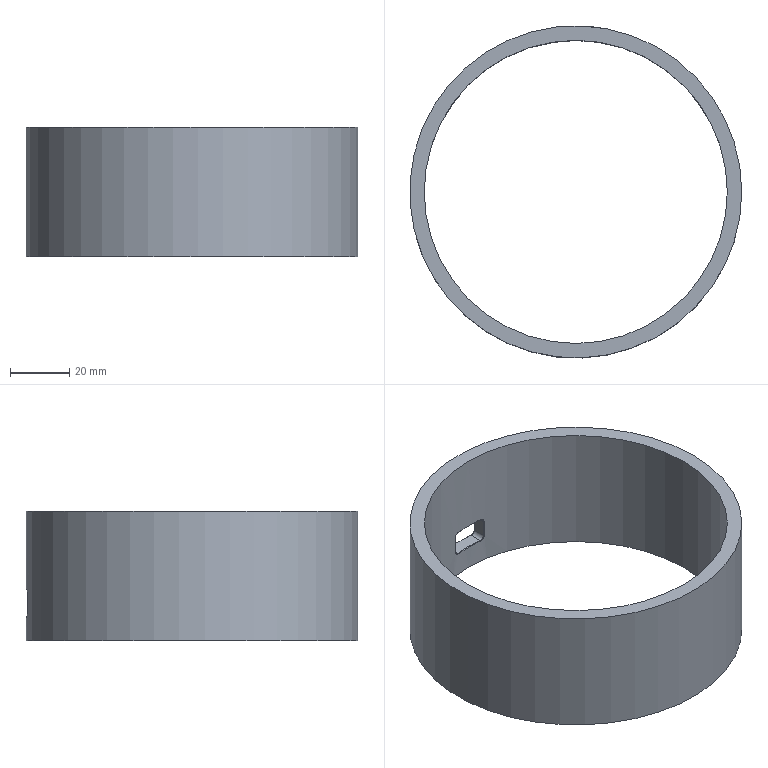Part | 1 solid | 28 faces | box 112.5 x 112.5 x 44 mm | volume 72321 mm3 | plane 10 | spline 8 | cylinder 6 | cone 4 | commonest cylinder face diameters 3 x4 102.7 x1 112.5 x1
STEP:
#1=CARTESIAN_POINT('',(-7.25,55.781,-28.5));
#2=VERTEX_POINT('',#1);
#3=CARTESIAN_POINT('',(-7.25,55.781,-34.));
#4=VERTEX_POINT('',#3);
#5=CARTESIAN_POINT('',(-7.25,55.781,0.));
#6=DIRECTION('',(0.,0.,-1.));
#7=VECTOR('',#6,1000.);
#8=LINE('',#5,#7);
#9=EDGE_CURVE('',#2,#4,#8,.T.);
#10=ORIENTED_EDGE('',*,*,#9,.T.);
#11=CARTESIAN_POINT('',(-5.292,56.001,-35.943));
#12=VERTEX_POINT('',#11);
#13=CARTESIAN_POINT('',(-7.25,55.781,-34.));
#14=CARTESIAN_POINT('',(-7.25,55.781,-35.034));
#15=CARTESIAN_POINT('',(-6.327,55.903,-35.945));
#16=CARTESIAN_POINT('',(-5.292,56.001,-35.943));
#17=B_SPLINE_CURVE_WITH_KNOTS('',3,(#13,#14,#15,#16),.UNSPECIFIED.,.F.,.F.,(4,4),(0.,1.),.UNSPECIFIED.);
#18=EDGE_CURVE('',#4,#12,#17,.T.);
#19=ORIENTED_EDGE('',*,*,#18,.T.);
#20=CARTESIAN_POINT('',(5.292,56.001,-35.943));
#21=VERTEX_POINT('',#20);
#22=CARTESIAN_POINT('',(0.,0.,-35.943));
#23=DIRECTION('',(0.,0.,1.));
#24=DIRECTION('',(1.,0.,0.));
#25=AXIS2_PLACEMENT_3D('',#22,#23,#24);
#26=CIRCLE('',#25,56.25);
#27=EDGE_CURVE('',#12,#21,#26,.F.);
#28=ORIENTED_EDGE('',*,*,#27,.T.);
#29=CARTESIAN_POINT('',(7.25,55.781,-34.));
#30=VERTEX_POINT('',#29);
#31=CARTESIAN_POINT('',(5.292,56.001,-35.943));
#32=CARTESIAN_POINT('',(6.33,55.902,-35.943));
#33=CARTESIAN_POINT('',(7.252,55.781,-35.032));
#34=CARTESIAN_POINT('',(7.25,55.781,-34.));
#35=B_SPLINE_CURVE_WITH_KNOTS('',3,(#31,#32,#33,#34),.UNSPECIFIED.,.F.,.F.,(4,4),(0.,1.),.UNSPECIFIED.);
#36=EDGE_CURVE('',#21,#30,#35,.T.);
#37=ORIENTED_EDGE('',*,*,#36,.T.);
#38=CARTESIAN_POINT('',(7.25,55.781,-28.5));
#39=VERTEX_POINT('',#38);
#40=CARTESIAN_POINT('',(7.25,55.781,0.));
#41=DIRECTION('',(0.,0.,-1.));
#42=VECTOR('',#41,1000.);
#43=LINE('',#40,#42);
#44=EDGE_CURVE('',#30,#39,#43,.F.);
#45=ORIENTED_EDGE('',*,*,#44,.T.);
#46=CARTESIAN_POINT('',(5.292,56.001,-26.557));
#47=VERTEX_POINT('',#46);
#48=CARTESIAN_POINT('',(7.25,55.781,-28.5));
#49=CARTESIAN_POINT('',(7.25,55.781,-27.466));
#50=CARTESIAN_POINT('',(6.327,55.903,-26.555));
#51=CARTESIAN_POINT('',(5.292,56.001,-26.557));
#52=B_SPLINE_CURVE_WITH_KNOTS('',3,(#48,#49,#50,#51),.UNSPECIFIED.,.F.,.F.,(4,4),(0.,1.),.UNSPECIFIED.);
#53=EDGE_CURVE('',#39,#47,#52,.T.);
#54=ORIENTED_EDGE('',*,*,#53,.T.);
#55=CARTESIAN_POINT('',(-5.292,56.001,-26.557));
#56=VERTEX_POINT('',#55);
#57=CARTESIAN_POINT('',(0.,0.,-26.557));
#58=DIRECTION('',(0.,0.,-1.));
#59=DIRECTION('',(-1.,0.,0.));
#60=AXIS2_PLACEMENT_3D('',#57,#58,#59);
#61=CIRCLE('',#60,56.25);
#62=EDGE_CURVE('',#47,#56,#61,.F.);
#63=ORIENTED_EDGE('',*,*,#62,.T.);
#64=CARTESIAN_POINT('',(-5.292,56.001,-26.557));
#65=CARTESIAN_POINT('',(-6.33,55.902,-26.557));
#66=CARTESIAN_POINT('',(-7.252,55.781,-27.468));
#67=CARTESIAN_POINT('',(-7.25,55.781,-28.5));
#68=B_SPLINE_CURVE_WITH_KNOTS('',3,(#64,#65,#66,#67),.UNSPECIFIED.,.F.,.F.,(4,4),(0.,1.),.UNSPECIFIED.);
#69=EDGE_CURVE('',#56,#2,#68,.T.);
#70=ORIENTED_EDGE('',*,*,#69,.T.);
#71=EDGE_LOOP('',(#10,#19,#28,#37,#45,#54,#63,#70));
#72=FACE_BOUND('',#71,.T.);
#73=CARTESIAN_POINT('',(56.25,0.,0.));
#74=VERTEX_POINT('',#73);
#75=CARTESIAN_POINT('',(0.,0.,0.));
#76=DIRECTION('',(0.,0.,1.));
#77=DIRECTION('',(1.,0.,0.));
#78=AXIS2_PLACEMENT_3D('',#75,#76,#77);
#79=CIRCLE('',#78,56.25);
#80=EDGE_CURVE('',#74,#74,#79,.T.);
#81=ORIENTED_EDGE('',*,*,#80,.F.);
#82=EDGE_LOOP('',(#81));
#83=FACE_BOUND('',#82,.T.);
#84=CARTESIAN_POINT('',(56.25,0.,-44.));
#85=VERTEX_POINT('',#84);
#86=CARTESIAN_POINT('',(0.,0.,-44.));
#87=DIRECTION('',(0.,0.,1.));
#88=DIRECTION('',(1.,0.,0.));
#89=AXIS2_PLACEMENT_3D('',#86,#87,#88);
#90=CIRCLE('',#89,56.25);
#91=EDGE_CURVE('',#85,#85,#90,.T.);
#92=ORIENTED_EDGE('',*,*,#91,.T.);
#93=EDGE_LOOP('',(#92));
#94=FACE_BOUND('',#93,.T.);
#95=CARTESIAN_POINT('',(0.,0.,0.));
#96=DIRECTION('',(0.,0.,-1.));
#97=DIRECTION('',(-1.,0.,0.));
#98=AXIS2_PLACEMENT_3D('',#95,#96,#97);
#99=CYLINDRICAL_SURFACE('',#98,56.25);
#100=ADVANCED_FACE('',(#72,#83,#94),#99,.T.);
#101=CARTESIAN_POINT('',(-6.923,50.881,-34.));
#102=VERTEX_POINT('',#101);
#103=CARTESIAN_POINT('',(-6.923,50.881,-28.5));
#104=VERTEX_POINT('',#103);
#105=CARTESIAN_POINT('',(-6.923,50.881,0.));
#106=DIRECTION('',(0.,0.,-1.));
#107=VECTOR('',#106,1000.);
#108=LINE('',#105,#107);
#109=EDGE_CURVE('',#102,#104,#108,.F.);
#110=ORIENTED_EDGE('',*,*,#109,.T.);
#111=CARTESIAN_POINT('',(-5.23,51.083,-26.8));
#112=VERTEX_POINT('',#111);
#113=CARTESIAN_POINT('',(-6.923,50.881,-28.5));
#114=CARTESIAN_POINT('',(-6.924,50.881,-27.597));
#115=CARTESIAN_POINT('',(-6.126,50.991,-26.801));
#116=CARTESIAN_POINT('',(-5.23,51.083,-26.8));
#117=B_SPLINE_CURVE_WITH_KNOTS('',3,(#113,#114,#115,#116),.UNSPECIFIED.,.F.,.F.,(4,4),(0.,1.),.UNSPECIFIED.);
#118=EDGE_CURVE('',#104,#112,#117,.T.);
#119=ORIENTED_EDGE('',*,*,#118,.T.);
#120=CARTESIAN_POINT('',(5.23,51.083,-26.8));
#121=VERTEX_POINT('',#120);
#122=CARTESIAN_POINT('',(0.,0.,-26.8));
#123=DIRECTION('',(0.,0.,-1.));
#124=DIRECTION('',(-1.,0.,0.));
#125=AXIS2_PLACEMENT_3D('',#122,#123,#124);
#126=CIRCLE('',#125,51.35);
#127=EDGE_CURVE('',#112,#121,#126,.T.);
#128=ORIENTED_EDGE('',*,*,#127,.T.);
#129=CARTESIAN_POINT('',(6.923,50.881,-28.5));
#130=VERTEX_POINT('',#129);
#131=CARTESIAN_POINT('',(5.23,51.083,-26.8));
#132=CARTESIAN_POINT('',(6.118,50.992,-26.797));
#133=CARTESIAN_POINT('',(6.923,50.881,-27.596));
#134=CARTESIAN_POINT('',(6.923,50.881,-28.5));
#135=B_SPLINE_CURVE_WITH_KNOTS('',3,(#131,#132,#133,#134),.UNSPECIFIED.,.F.,.F.,(4,4),(0.,1.),.UNSPECIFIED.);
#136=EDGE_CURVE('',#121,#130,#135,.T.);
#137=ORIENTED_EDGE('',*,*,#136,.T.);
#138=CARTESIAN_POINT('',(6.923,50.881,-34.));
#139=VERTEX_POINT('',#138);
#140=CARTESIAN_POINT('',(6.923,50.881,0.));
#141=DIRECTION('',(0.,0.,-1.));
#142=VECTOR('',#141,1000.);
#143=LINE('',#140,#142);
#144=EDGE_CURVE('',#130,#139,#143,.T.);
#145=ORIENTED_EDGE('',*,*,#144,.T.);
#146=CARTESIAN_POINT('',(5.23,51.083,-35.7));
#147=VERTEX_POINT('',#146);
#148=CARTESIAN_POINT('',(6.923,50.881,-34.));
#149=CARTESIAN_POINT('',(6.924,50.881,-34.903));
#150=CARTESIAN_POINT('',(6.126,50.991,-35.699));
#151=CARTESIAN_POINT('',(5.23,51.083,-35.7));
#152=B_SPLINE_CURVE_WITH_KNOTS('',3,(#148,#149,#150,#151),.UNSPECIFIED.,.F.,.F.,(4,4),(0.,1.),.UNSPECIFIED.);
#153=EDGE_CURVE('',#139,#147,#152,.T.);
#154=ORIENTED_EDGE('',*,*,#153,.T.);
#155=CARTESIAN_POINT('',(-5.23,51.083,-35.7));
#156=VERTEX_POINT('',#155);
#157=CARTESIAN_POINT('',(0.,0.,-35.7));
#158=DIRECTION('',(0.,0.,1.));
#159=DIRECTION('',(1.,0.,0.));
#160=AXIS2_PLACEMENT_3D('',#157,#158,#159);
#161=CIRCLE('',#160,51.35);
#162=EDGE_CURVE('',#147,#156,#161,.T.);
#163=ORIENTED_EDGE('',*,*,#162,.T.);
#164=CARTESIAN_POINT('',(-5.23,51.083,-35.7));
#165=CARTESIAN_POINT('',(-6.118,50.992,-35.703));
#166=CARTESIAN_POINT('',(-6.923,50.881,-34.904));
#167=CARTESIAN_POINT('',(-6.923,50.881,-34.));
#168=B_SPLINE_CURVE_WITH_KNOTS('',3,(#164,#165,#166,#167),.UNSPECIFIED.,.F.,.F.,(4,4),(0.,1.),.UNSPECIFIED.);
#169=EDGE_CURVE('',#156,#102,#168,.T.);
#170=ORIENTED_EDGE('',*,*,#169,.T.);
#171=EDGE_LOOP('',(#110,#119,#128,#137,#145,#154,#163,#170));
#172=FACE_BOUND('',#171,.T.);
#173=CARTESIAN_POINT('',(51.35,0.,0.));
#174=VERTEX_POINT('',#173);
#175=CARTESIAN_POINT('',(0.,0.,0.));
#176=DIRECTION('',(0.,0.,1.));
#177=DIRECTION('',(1.,0.,0.));
#178=AXIS2_PLACEMENT_3D('',#175,#176,#177);
#179=CIRCLE('',#178,51.35);
#180=EDGE_CURVE('',#174,#174,#179,.T.);
#181=ORIENTED_EDGE('',*,*,#180,.T.);
#182=EDGE_LOOP('',(#181));
#183=FACE_BOUND('',#182,.T.);
#184=CARTESIAN_POINT('',(51.35,0.,-44.));
#185=VERTEX_POINT('',#184);
#186=CARTESIAN_POINT('',(0.,0.,-44.));
#187=DIRECTION('',(0.,0.,1.));
#188=DIRECTION('',(1.,0.,0.));
#189=AXIS2_PLACEMENT_3D('',#186,#187,#188);
#190=CIRCLE('',#189,51.35);
#191=EDGE_CURVE('',#185,#185,#190,.T.);
#192=ORIENTED_EDGE('',*,*,#191,.F.);
#193=EDGE_LOOP('',(#192));
#194=FACE_BOUND('',#193,.T.);
#195=CARTESIAN_POINT('',(0.,0.,0.));
#196=DIRECTION('',(0.,0.,-1.));
#197=DIRECTION('',(-1.,0.,0.));
#198=AXIS2_PLACEMENT_3D('',#195,#196,#197);
#199=CYLINDRICAL_SURFACE('',#198,51.35);
#200=ADVANCED_FACE('',(#172,#183,#194),#199,.F.);
#201=ORIENTED_EDGE('',*,*,#80,.T.);
#202=EDGE_LOOP('',(#201));
#203=FACE_BOUND('',#202,.T.);
#204=ORIENTED_EDGE('',*,*,#180,.F.);
#205=EDGE_LOOP('',(#204));
#206=FACE_BOUND('',#205,.T.);
#207=CARTESIAN_POINT('',(0.,0.,0.));
#208=DIRECTION('',(0.,0.,1.));
#209=DIRECTION('',(1.,0.,0.));
#210=AXIS2_PLACEMENT_3D('',#207,#208,#209);
#211=PLANE('',#210);
#212=ADVANCED_FACE('',(#203,#206),#211,.T.);
#213=ORIENTED_EDGE('',*,*,#91,.F.);
#214=EDGE_LOOP('',(#213));
#215=FACE_BOUND('',#214,.T.);
#216=ORIENTED_EDGE('',*,*,#191,.T.);
#217=EDGE_LOOP('',(#216));
#218=FACE_BOUND('',#217,.T.);
#219=CARTESIAN_POINT('',(0.,0.,-44.));
#220=DIRECTION('',(0.,0.,1.));
#221=DIRECTION('',(1.,0.,0.));
#222=AXIS2_PLACEMENT_3D('',#219,#220,#221);
#223=PLANE('',#222);
#224=ADVANCED_FACE('',(#215,#218),#223,.F.);
#225=CARTESIAN_POINT('',(-6.75,55.341,-28.5));
#226=VERTEX_POINT('',#225);
#227=CARTESIAN_POINT('',(-6.75,51.079,-28.5));
#228=VERTEX_POINT('',#227);
#229=CARTESIAN_POINT('',(-6.75,50.904,-28.5));
#230=DIRECTION('',(0.,1.,0.));
#231=VECTOR('',#230,1000.);
#232=LINE('',#229,#231);
#233=EDGE_CURVE('',#226,#228,#232,.F.);
#234=ORIENTED_EDGE('',*,*,#233,.T.);
#235=CARTESIAN_POINT('',(-6.75,51.079,-34.));
#236=VERTEX_POINT('',#235);
#237=CARTESIAN_POINT('',(-6.75,51.079,-35.5));
#238=DIRECTION('',(0.,0.,-1.));
#239=VECTOR('',#238,1000.);
#240=LINE('',#237,#239);
#241=EDGE_CURVE('',#228,#236,#240,.T.);
#242=ORIENTED_EDGE('',*,*,#241,.T.);
#243=CARTESIAN_POINT('',(-6.75,55.341,-34.));
#244=VERTEX_POINT('',#243);
#245=CARTESIAN_POINT('',(-6.75,55.844,-34.));
#246=DIRECTION('',(0.,1.,0.));
#247=VECTOR('',#246,1000.);
#248=LINE('',#245,#247);
#249=EDGE_CURVE('',#236,#244,#248,.T.);
#250=ORIENTED_EDGE('',*,*,#249,.T.);
#251=CARTESIAN_POINT('',(-6.75,55.341,-28.5));
#252=DIRECTION('',(0.,0.,1.));
#253=VECTOR('',#252,1000.);
#254=LINE('',#251,#253);
#255=EDGE_CURVE('',#244,#226,#254,.T.);
#256=ORIENTED_EDGE('',*,*,#255,.T.);
#257=EDGE_LOOP('',(#234,#242,#250,#256));
#258=FACE_BOUND('',#257,.T.);
#259=CARTESIAN_POINT('',(-6.75,56.25,-35.5));
#260=DIRECTION('',(1.,0.,0.));
#261=DIRECTION('',(0.,0.,-1.));
#262=AXIS2_PLACEMENT_3D('',#259,#260,#261);
#263=PLANE('',#262);
#264=ADVANCED_FACE('',(#258),#263,.T.);
#265=CARTESIAN_POINT('',(5.25,55.559,-27.));
#266=VERTEX_POINT('',#265);
#267=CARTESIAN_POINT('',(5.25,51.282,-27.));
#268=VERTEX_POINT('',#267);
#269=CARTESIAN_POINT('',(5.25,50.904,-27.));
#270=DIRECTION('',(0.,1.,0.));
#271=VECTOR('',#270,1000.);
#272=LINE('',#269,#271);
#273=EDGE_CURVE('',#266,#268,#272,.F.);
#274=ORIENTED_EDGE('',*,*,#273,.T.);
#275=CARTESIAN_POINT('',(-5.25,51.282,-27.));
#276=VERTEX_POINT('',#275);
#277=CARTESIAN_POINT('',(0.,0.,-27.));
#278=DIRECTION('',(0.,0.,-1.));
#279=DIRECTION('',(-1.,0.,0.));
#280=AXIS2_PLACEMENT_3D('',#277,#278,#279);
#281=CIRCLE('',#280,51.55);
#282=EDGE_CURVE('',#268,#276,#281,.F.);
#283=ORIENTED_EDGE('',*,*,#282,.T.);
#284=CARTESIAN_POINT('',(-5.25,55.559,-27.));
#285=VERTEX_POINT('',#284);
#286=CARTESIAN_POINT('',(-5.25,55.844,-27.));
#287=DIRECTION('',(0.,1.,0.));
#288=VECTOR('',#287,1000.);
#289=LINE('',#286,#288);
#290=EDGE_CURVE('',#276,#285,#289,.T.);
#291=ORIENTED_EDGE('',*,*,#290,.T.);
#292=CARTESIAN_POINT('',(0.,0.,-27.));
#293=DIRECTION('',(0.,0.,-1.));
#294=DIRECTION('',(-1.,0.,0.));
#295=AXIS2_PLACEMENT_3D('',#292,#293,#294);
#296=CIRCLE('',#295,55.807);
#297=EDGE_CURVE('',#285,#266,#296,.T.);
#298=ORIENTED_EDGE('',*,*,#297,.T.);
#299=EDGE_LOOP('',(#274,#283,#291,#298));
#300=FACE_BOUND('',#299,.T.);
#301=CARTESIAN_POINT('',(-6.75,56.25,-27.));
#302=DIRECTION('',(0.,0.,-1.));
#303=DIRECTION('',(-1.,0.,0.));
#304=AXIS2_PLACEMENT_3D('',#301,#302,#303);
#305=PLANE('',#304);
#306=ADVANCED_FACE('',(#300),#305,.T.);
#307=CARTESIAN_POINT('',(6.75,55.341,-34.));
#308=VERTEX_POINT('',#307);
#309=CARTESIAN_POINT('',(6.75,51.079,-34.));
#310=VERTEX_POINT('',#309);
#311=CARTESIAN_POINT('',(6.75,50.904,-34.));
#312=DIRECTION('',(0.,1.,0.));
#313=VECTOR('',#312,1000.);
#314=LINE('',#311,#313);
#315=EDGE_CURVE('',#308,#310,#314,.F.);
#316=ORIENTED_EDGE('',*,*,#315,.T.);
#317=CARTESIAN_POINT('',(6.75,51.079,-28.5));
#318=VERTEX_POINT('',#317);
#319=CARTESIAN_POINT('',(6.75,51.079,-27.));
#320=DIRECTION('',(0.,0.,1.));
#321=VECTOR('',#320,1000.);
#322=LINE('',#319,#321);
#323=EDGE_CURVE('',#310,#318,#322,.T.);
#324=ORIENTED_EDGE('',*,*,#323,.T.);
#325=CARTESIAN_POINT('',(6.75,55.341,-28.5));
#326=VERTEX_POINT('',#325);
#327=CARTESIAN_POINT('',(6.75,55.844,-28.5));
#328=DIRECTION('',(0.,1.,0.));
#329=VECTOR('',#328,1000.);
#330=LINE('',#327,#329);
#331=EDGE_CURVE('',#318,#326,#330,.T.);
#332=ORIENTED_EDGE('',*,*,#331,.T.);
#333=CARTESIAN_POINT('',(6.75,55.341,-34.));
#334=DIRECTION('',(0.,0.,-1.));
#335=VECTOR('',#334,1000.);
#336=LINE('',#333,#335);
#337=EDGE_CURVE('',#326,#308,#336,.T.);
#338=ORIENTED_EDGE('',*,*,#337,.T.);
#339=EDGE_LOOP('',(#316,#324,#332,#338));
#340=FACE_BOUND('',#339,.T.);
#341=CARTESIAN_POINT('',(6.75,56.25,-27.));
#342=DIRECTION('',(-1.,0.,0.));
#343=DIRECTION('',(0.,0.,1.));
#344=AXIS2_PLACEMENT_3D('',#341,#342,#343);
#345=PLANE('',#344);
#346=ADVANCED_FACE('',(#340),#345,.T.);
#347=CARTESIAN_POINT('',(-5.25,55.559,-35.5));
#348=VERTEX_POINT('',#347);
#349=CARTESIAN_POINT('',(-5.25,51.282,-35.5));
#350=VERTEX_POINT('',#349);
#351=CARTESIAN_POINT('',(-5.25,50.904,-35.5));
#352=DIRECTION('',(0.,1.,0.));
#353=VECTOR('',#352,1000.);
#354=LINE('',#351,#353);
#355=EDGE_CURVE('',#348,#350,#354,.F.);
#356=ORIENTED_EDGE('',*,*,#355,.T.);
#357=CARTESIAN_POINT('',(5.25,51.282,-35.5));
#358=VERTEX_POINT('',#357);
#359=CARTESIAN_POINT('',(0.,0.,-35.5));
#360=DIRECTION('',(0.,0.,1.));
#361=DIRECTION('',(1.,0.,0.));
#362=AXIS2_PLACEMENT_3D('',#359,#360,#361);
#363=CIRCLE('',#362,51.55);
#364=EDGE_CURVE('',#350,#358,#363,.F.);
#365=ORIENTED_EDGE('',*,*,#364,.T.);
#366=CARTESIAN_POINT('',(5.25,55.559,-35.5));
#367=VERTEX_POINT('',#366);
#368=CARTESIAN_POINT('',(5.25,55.844,-35.5));
#369=DIRECTION('',(0.,1.,0.));
#370=VECTOR('',#369,1000.);
#371=LINE('',#368,#370);
#372=EDGE_CURVE('',#358,#367,#371,.T.);
#373=ORIENTED_EDGE('',*,*,#372,.T.);
#374=CARTESIAN_POINT('',(0.,0.,-35.5));
#375=DIRECTION('',(0.,0.,1.));
#376=DIRECTION('',(1.,0.,0.));
#377=AXIS2_PLACEMENT_3D('',#374,#375,#376);
#378=CIRCLE('',#377,55.807);
#379=EDGE_CURVE('',#367,#348,#378,.T.);
#380=ORIENTED_EDGE('',*,*,#379,.T.);
#381=EDGE_LOOP('',(#356,#365,#373,#380));
#382=FACE_BOUND('',#381,.T.);
#383=CARTESIAN_POINT('',(6.75,56.25,-35.5));
#384=DIRECTION('',(0.,0.,1.));
#385=DIRECTION('',(1.,0.,0.));
#386=AXIS2_PLACEMENT_3D('',#383,#384,#385);
#387=PLANE('',#386);
#388=ADVANCED_FACE('',(#382),#387,.T.);
#389=ORIENTED_EDGE('',*,*,#372,.F.);
#390=CARTESIAN_POINT('',(5.25,51.282,-35.5));
#391=CARTESIAN_POINT('',(5.272,51.279,-35.5));
#392=CARTESIAN_POINT('',(5.374,51.268,-35.513));
#393=CARTESIAN_POINT('',(6.019,51.187,-35.347));
#394=CARTESIAN_POINT('',(6.297,51.146,-35.109));
#395=CARTESIAN_POINT('',(6.702,51.088,-34.547));
#396=CARTESIAN_POINT('',(6.75,51.079,-34.177));
#397=CARTESIAN_POINT('',(6.75,51.079,-34.));
#398=B_SPLINE_CURVE_WITH_KNOTS('',3,(#390,#391,#392,#393,#394,#395,#396,#397),.UNSPECIFIED.,.F.,.F.,(4,1,1,1,1,4),(0.,0.125,0.25,0.5,0.75,1.),.UNSPECIFIED.);
#399=EDGE_CURVE('',#358,#310,#398,.T.);
#400=ORIENTED_EDGE('',*,*,#399,.T.);
#401=ORIENTED_EDGE('',*,*,#315,.F.);
#402=CARTESIAN_POINT('',(6.75,55.341,-34.));
#403=CARTESIAN_POINT('',(6.75,55.341,-34.176));
#404=CARTESIAN_POINT('',(6.702,55.351,-34.539));
#405=CARTESIAN_POINT('',(6.365,55.404,-35.031));
#406=CARTESIAN_POINT('',(6.128,55.44,-35.223));
#407=CARTESIAN_POINT('',(5.847,55.482,-35.398));
#408=CARTESIAN_POINT('',(5.42,55.538,-35.504));
#409=CARTESIAN_POINT('',(5.292,55.554,-35.5));
#410=CARTESIAN_POINT('',(5.25,55.559,-35.5));
#411=B_SPLINE_CURVE_WITH_KNOTS('',3,(#402,#403,#404,#405,#406,#407,#408,#409,#410),.UNSPECIFIED.,.F.,.F.,(4,1,1,1,1,1,4),(0.,0.25,0.5,0.625,0.75,0.875,1.),.UNSPECIFIED.);
#412=EDGE_CURVE('',#308,#367,#411,.T.);
#413=ORIENTED_EDGE('',*,*,#412,.T.);
#414=EDGE_LOOP('',(#389,#400,#401,#413));
#415=FACE_BOUND('',#414,.T.);
#416=CARTESIAN_POINT('',(5.25,56.25,-34.));
#417=DIRECTION('',(0.,-1.,0.));
#418=DIRECTION('',(0.,0.,-1.));
#419=AXIS2_PLACEMENT_3D('',#416,#417,#418);
#420=CYLINDRICAL_SURFACE('',#419,1.5);
#421=ADVANCED_FACE('',(#415),#420,.F.);
#422=ORIENTED_EDGE('',*,*,#331,.F.);
#423=CARTESIAN_POINT('',(6.75,51.079,-28.5));
#424=CARTESIAN_POINT('',(6.75,51.079,-28.322));
#425=CARTESIAN_POINT('',(6.702,51.088,-27.951));
#426=CARTESIAN_POINT('',(6.295,51.147,-27.392));
#427=CARTESIAN_POINT('',(6.029,51.186,-27.155));
#428=CARTESIAN_POINT('',(5.36,51.269,-26.984));
#429=CARTESIAN_POINT('',(5.266,51.28,-27.));
#430=CARTESIAN_POINT('',(5.25,51.282,-27.));
#431=B_SPLINE_CURVE_WITH_KNOTS('',3,(#423,#424,#425,#426,#427,#428,#429,#430),.UNSPECIFIED.,.F.,.F.,(4,1,1,1,1,4),(0.,0.25,0.5,0.75,0.875,1.),.UNSPECIFIED.);
#432=EDGE_CURVE('',#318,#268,#431,.T.);
#433=ORIENTED_EDGE('',*,*,#432,.T.);
#434=ORIENTED_EDGE('',*,*,#273,.F.);
#435=CARTESIAN_POINT('',(5.25,55.559,-27.));
#436=CARTESIAN_POINT('',(5.292,55.554,-27.));
#437=CARTESIAN_POINT('',(5.419,55.538,-26.996));
#438=CARTESIAN_POINT('',(5.849,55.481,-27.103));
#439=CARTESIAN_POINT('',(6.128,55.44,-27.277));
#440=CARTESIAN_POINT('',(6.367,55.404,-27.47));
#441=CARTESIAN_POINT('',(6.701,55.351,-27.96));
#442=CARTESIAN_POINT('',(6.75,55.341,-28.323));
#443=CARTESIAN_POINT('',(6.75,55.341,-28.5));
#444=B_SPLINE_CURVE_WITH_KNOTS('',3,(#435,#436,#437,#438,#439,#440,#441,#442,#443),.UNSPECIFIED.,.F.,.F.,(4,1,1,1,1,1,4),(0.,0.125,0.25,0.375,0.5,0.75,1.),.UNSPECIFIED.);
#445=EDGE_CURVE('',#266,#326,#444,.T.);
#446=ORIENTED_EDGE('',*,*,#445,.T.);
#447=EDGE_LOOP('',(#422,#433,#434,#446));
#448=FACE_BOUND('',#447,.T.);
#449=CARTESIAN_POINT('',(5.25,56.25,-28.5));
#450=DIRECTION('',(0.,-1.,0.));
#451=DIRECTION('',(0.,0.,-1.));
#452=AXIS2_PLACEMENT_3D('',#449,#450,#451);
#453=CYLINDRICAL_SURFACE('',#452,1.5);
#454=ADVANCED_FACE('',(#448),#453,.F.);
#455=ORIENTED_EDGE('',*,*,#290,.F.);
#456=CARTESIAN_POINT('',(-5.25,51.282,-27.));
#457=CARTESIAN_POINT('',(-5.272,51.279,-27.));
#458=CARTESIAN_POINT('',(-5.374,51.268,-26.987));
#459=CARTESIAN_POINT('',(-6.019,51.187,-27.153));
#460=CARTESIAN_POINT('',(-6.297,51.146,-27.391));
#461=CARTESIAN_POINT('',(-6.702,51.088,-27.953));
#462=CARTESIAN_POINT('',(-6.75,51.079,-28.323));
#463=CARTESIAN_POINT('',(-6.75,51.079,-28.5));
#464=B_SPLINE_CURVE_WITH_KNOTS('',3,(#456,#457,#458,#459,#460,#461,#462,#463),.UNSPECIFIED.,.F.,.F.,(4,1,1,1,1,4),(0.,0.125,0.25,0.5,0.75,1.),.UNSPECIFIED.);
#465=EDGE_CURVE('',#276,#228,#464,.T.);
#466=ORIENTED_EDGE('',*,*,#465,.T.);
#467=ORIENTED_EDGE('',*,*,#233,.F.);
#468=CARTESIAN_POINT('',(-6.75,55.341,-28.5));
#469=CARTESIAN_POINT('',(-6.75,55.341,-28.324));
#470=CARTESIAN_POINT('',(-6.702,55.351,-27.961));
#471=CARTESIAN_POINT('',(-6.365,55.404,-27.469));
#472=CARTESIAN_POINT('',(-6.128,55.44,-27.277));
#473=CARTESIAN_POINT('',(-5.847,55.482,-27.102));
#474=CARTESIAN_POINT('',(-5.42,55.538,-26.996));
#475=CARTESIAN_POINT('',(-5.292,55.554,-27.));
#476=CARTESIAN_POINT('',(-5.25,55.559,-27.));
#477=B_SPLINE_CURVE_WITH_KNOTS('',3,(#468,#469,#470,#471,#472,#473,#474,#475,#476),.UNSPECIFIED.,.F.,.F.,(4,1,1,1,1,1,4),(0.,0.25,0.5,0.625,0.75,0.875,1.),.UNSPECIFIED.);
#478=EDGE_CURVE('',#226,#285,#477,.T.);
#479=ORIENTED_EDGE('',*,*,#478,.T.);
#480=EDGE_LOOP('',(#455,#466,#467,#479));
#481=FACE_BOUND('',#480,.T.);
#482=CARTESIAN_POINT('',(-5.25,56.25,-28.5));
#483=DIRECTION('',(0.,-1.,0.));
#484=DIRECTION('',(0.,0.,-1.));
#485=AXIS2_PLACEMENT_3D('',#482,#483,#484);
#486=CYLINDRICAL_SURFACE('',#485,1.5);
#487=ADVANCED_FACE('',(#481),#486,.F.);
#488=ORIENTED_EDGE('',*,*,#249,.F.);
#489=CARTESIAN_POINT('',(-6.75,51.079,-34.));
#490=CARTESIAN_POINT('',(-6.75,51.079,-34.178));
#491=CARTESIAN_POINT('',(-6.702,51.088,-34.549));
#492=CARTESIAN_POINT('',(-6.295,51.147,-35.108));
#493=CARTESIAN_POINT('',(-6.029,51.186,-35.345));
#494=CARTESIAN_POINT('',(-5.36,51.269,-35.516));
#495=CARTESIAN_POINT('',(-5.266,51.28,-35.5));
#496=CARTESIAN_POINT('',(-5.25,51.282,-35.5));
#497=B_SPLINE_CURVE_WITH_KNOTS('',3,(#489,#490,#491,#492,#493,#494,#495,#496),.UNSPECIFIED.,.F.,.F.,(4,1,1,1,1,4),(0.,0.25,0.5,0.75,0.875,1.),.UNSPECIFIED.);
#498=EDGE_CURVE('',#236,#350,#497,.T.);
#499=ORIENTED_EDGE('',*,*,#498,.T.);
#500=ORIENTED_EDGE('',*,*,#355,.F.);
#501=CARTESIAN_POINT('',(-5.25,55.559,-35.5));
#502=CARTESIAN_POINT('',(-5.292,55.554,-35.5));
#503=CARTESIAN_POINT('',(-5.419,55.538,-35.504));
#504=CARTESIAN_POINT('',(-5.849,55.481,-35.397));
#505=CARTESIAN_POINT('',(-6.128,55.44,-35.223));
#506=CARTESIAN_POINT('',(-6.367,55.404,-35.03));
#507=CARTESIAN_POINT('',(-6.701,55.351,-34.54));
#508=CARTESIAN_POINT('',(-6.75,55.341,-34.177));
#509=CARTESIAN_POINT('',(-6.75,55.341,-34.));
#510=B_SPLINE_CURVE_WITH_KNOTS('',3,(#501,#502,#503,#504,#505,#506,#507,#508,#509),.UNSPECIFIED.,.F.,.F.,(4,1,1,1,1,1,4),(0.,0.125,0.25,0.375,0.5,0.75,1.),.UNSPECIFIED.);
#511=EDGE_CURVE('',#348,#244,#510,.T.);
#512=ORIENTED_EDGE('',*,*,#511,.T.);
#513=EDGE_LOOP('',(#488,#499,#500,#512));
#514=FACE_BOUND('',#513,.T.);
#515=CARTESIAN_POINT('',(-5.25,56.25,-34.));
#516=DIRECTION('',(0.,-1.,0.));
#517=DIRECTION('',(0.,0.,-1.));
#518=AXIS2_PLACEMENT_3D('',#515,#516,#517);
#519=CYLINDRICAL_SURFACE('',#518,1.5);
#520=ADVANCED_FACE('',(#514),#519,.F.);
#521=CARTESIAN_POINT('',(6.75,55.341,-28.5));
#522=CARTESIAN_POINT('',(6.917,55.488,-28.5));
#523=CARTESIAN_POINT('',(7.084,55.634,-28.5));
#524=CARTESIAN_POINT('',(7.25,55.781,-28.5));
#525=B_SPLINE_CURVE_WITH_KNOTS('',3,(#521,#522,#523,#524),.UNSPECIFIED.,.F.,.F.,(4,4),(0.,1.),.UNSPECIFIED.);
#526=EDGE_CURVE('',#326,#39,#525,.T.);
#527=ORIENTED_EDGE('',*,*,#526,.F.);
#528=ORIENTED_EDGE('',*,*,#445,.F.);
#529=CARTESIAN_POINT('',(5.292,56.001,-26.557));
#530=CARTESIAN_POINT('',(5.278,55.853,-26.705));
#531=CARTESIAN_POINT('',(5.264,55.706,-26.852));
#532=CARTESIAN_POINT('',(5.25,55.559,-27.));
#533=B_SPLINE_CURVE_WITH_KNOTS('',3,(#529,#530,#531,#532),.UNSPECIFIED.,.F.,.F.,(4,4),(0.,1.),.UNSPECIFIED.);
#534=EDGE_CURVE('',#47,#266,#533,.T.);
#535=ORIENTED_EDGE('',*,*,#534,.F.);
#536=ORIENTED_EDGE('',*,*,#53,.F.);
#537=EDGE_LOOP('',(#527,#528,#535,#536));
#538=FACE_BOUND('',#537,.T.);
#539=CARTESIAN_POINT('',(7.25,55.781,-28.5));
#540=CARTESIAN_POINT('',(7.25,55.781,-28.371));
#541=CARTESIAN_POINT('',(7.237,55.782,-28.245));
#542=CARTESIAN_POINT('',(7.188,55.789,-27.996));
#543=CARTESIAN_POINT('',(7.15,55.794,-27.872));
#544=CARTESIAN_POINT('',(7.051,55.806,-27.637));
#545=CARTESIAN_POINT('',(6.991,55.814,-27.525));
#546=CARTESIAN_POINT('',(6.849,55.832,-27.314));
#547=CARTESIAN_POINT('',(6.766,55.842,-27.214));
#548=CARTESIAN_POINT('',(6.495,55.874,-26.946));
#549=CARTESIAN_POINT('',(6.276,55.899,-26.801));
#550=CARTESIAN_POINT('',(5.807,55.95,-26.608));
#551=CARTESIAN_POINT('',(5.548,55.976,-26.556));
#552=CARTESIAN_POINT('',(5.292,56.001,-26.557));
#553=CARTESIAN_POINT('',(6.75,55.341,-28.5));
#554=CARTESIAN_POINT('',(6.75,55.341,-28.401));
#555=CARTESIAN_POINT('',(6.74,55.343,-28.303));
#556=CARTESIAN_POINT('',(6.702,55.349,-28.111));
#557=CARTESIAN_POINT('',(6.673,55.354,-28.016));
#558=CARTESIAN_POINT('',(6.597,55.367,-27.834));
#559=CARTESIAN_POINT('',(6.551,55.374,-27.748));
#560=CARTESIAN_POINT('',(6.442,55.392,-27.584));
#561=CARTESIAN_POINT('',(6.379,55.402,-27.507));
#562=CARTESIAN_POINT('',(6.172,55.434,-27.3));
#563=CARTESIAN_POINT('',(6.004,55.459,-27.189));
#564=CARTESIAN_POINT('',(5.644,55.509,-27.04));
#565=CARTESIAN_POINT('',(5.447,55.535,-27.));
#566=CARTESIAN_POINT('',(5.25,55.559,-27.));
#567=B_SPLINE_SURFACE_WITH_KNOTS('',1,3,((#539,#540,#541,#542,#543,#544,#545,#546,#547,#548,#549,#550,#551,#552),(#553,#554,#555,#556,#557,#558,#559,#560,#561,#562,#563,#564,#565,#566)),.RULED_SURF.,.F.,.F.,.F.,(2,2),(4,2,2,2,2,2,4),(0.,1.),(0.,0.0003806,0.0007612,0.001142,0.001522,0.002284,0.003045),.UNSPECIFIED.);
#568=ADVANCED_FACE('',(#538),#567,.T.);
#569=ORIENTED_EDGE('',*,*,#534,.T.);
#570=ORIENTED_EDGE('',*,*,#297,.F.);
#571=CARTESIAN_POINT('',(-5.25,55.559,-27.));
#572=CARTESIAN_POINT('',(-5.264,55.706,-26.852));
#573=CARTESIAN_POINT('',(-5.278,55.853,-26.705));
#574=CARTESIAN_POINT('',(-5.292,56.001,-26.557));
#575=B_SPLINE_CURVE_WITH_KNOTS('',3,(#571,#572,#573,#574),.UNSPECIFIED.,.F.,.F.,(4,4),(0.,1.),.UNSPECIFIED.);
#576=EDGE_CURVE('',#56,#285,#575,.F.);
#577=ORIENTED_EDGE('',*,*,#576,.F.);
#578=ORIENTED_EDGE('',*,*,#62,.F.);
#579=EDGE_LOOP('',(#569,#570,#577,#578));
#580=FACE_BOUND('',#579,.T.);
#581=CARTESIAN_POINT('',(0.,0.,-27.));
#582=DIRECTION('',(0.,0.,1.));
#583=DIRECTION('',(1.,0.,0.));
#584=AXIS2_PLACEMENT_3D('',#581,#582,#583);
#585=CONICAL_SURFACE('',#584,55.807,0.7854);
#586=ADVANCED_FACE('',(#580),#585,.T.);
#587=ORIENTED_EDGE('',*,*,#526,.T.);
#588=ORIENTED_EDGE('',*,*,#44,.F.);
#589=CARTESIAN_POINT('',(7.25,55.781,-34.));
#590=CARTESIAN_POINT('',(7.084,55.634,-34.));
#591=CARTESIAN_POINT('',(6.917,55.488,-34.));
#592=CARTESIAN_POINT('',(6.75,55.341,-34.));
#593=B_SPLINE_CURVE_WITH_KNOTS('',3,(#589,#590,#591,#592),.UNSPECIFIED.,.F.,.F.,(4,4),(0.,1.),.UNSPECIFIED.);
#594=EDGE_CURVE('',#308,#30,#593,.F.);
#595=ORIENTED_EDGE('',*,*,#594,.F.);
#596=ORIENTED_EDGE('',*,*,#337,.F.);
#597=EDGE_LOOP('',(#587,#588,#595,#596));
#598=FACE_BOUND('',#597,.T.);
#599=CARTESIAN_POINT('',(6.75,55.341,0.));
#600=DIRECTION('',(0.66,-0.7513,0.));
#601=DIRECTION('',(0.,0.,-1.));
#602=AXIS2_PLACEMENT_3D('',#599,#600,#601);
#603=PLANE('',#602);
#604=ADVANCED_FACE('',(#598),#603,.F.);
#605=ORIENTED_EDGE('',*,*,#576,.T.);
#606=ORIENTED_EDGE('',*,*,#478,.F.);
#607=CARTESIAN_POINT('',(-7.25,55.781,-28.5));
#608=CARTESIAN_POINT('',(-7.084,55.634,-28.5));
#609=CARTESIAN_POINT('',(-6.917,55.488,-28.5));
#610=CARTESIAN_POINT('',(-6.75,55.341,-28.5));
#611=B_SPLINE_CURVE_WITH_KNOTS('',3,(#607,#608,#609,#610),.UNSPECIFIED.,.F.,.F.,(4,4),(0.,1.),.UNSPECIFIED.);
#612=EDGE_CURVE('',#2,#226,#611,.T.);
#613=ORIENTED_EDGE('',*,*,#612,.F.);
#614=ORIENTED_EDGE('',*,*,#69,.F.);
#615=EDGE_LOOP('',(#605,#606,#613,#614));
#616=FACE_BOUND('',#615,.T.);
#617=CARTESIAN_POINT('',(-5.292,56.001,-26.557));
#618=CARTESIAN_POINT('',(-5.421,55.988,-26.557));
#619=CARTESIAN_POINT('',(-5.548,55.976,-26.569));
#620=CARTESIAN_POINT('',(-5.797,55.951,-26.618));
#621=CARTESIAN_POINT('',(-5.921,55.938,-26.656));
#622=CARTESIAN_POINT('',(-6.158,55.912,-26.753));
#623=CARTESIAN_POINT('',(-6.271,55.899,-26.812));
#624=CARTESIAN_POINT('',(-6.483,55.875,-26.952));
#625=CARTESIAN_POINT('',(-6.584,55.863,-27.034));
#626=CARTESIAN_POINT('',(-6.765,55.842,-27.213));
#627=CARTESIAN_POINT('',(-6.846,55.832,-27.31));
#628=CARTESIAN_POINT('',(-6.99,55.814,-27.523));
#629=CARTESIAN_POINT('',(-7.051,55.806,-27.636));
#630=CARTESIAN_POINT('',(-7.198,55.788,-27.987));
#631=CARTESIAN_POINT('',(-7.251,55.781,-28.244));
#632=CARTESIAN_POINT('',(-7.25,55.781,-28.5));
#633=CARTESIAN_POINT('',(-5.25,55.559,-27.));
#634=CARTESIAN_POINT('',(-5.349,55.547,-27.));
#635=CARTESIAN_POINT('',(-5.446,55.535,-27.01));
#636=CARTESIAN_POINT('',(-5.637,55.51,-27.048));
#637=CARTESIAN_POINT('',(-5.732,55.497,-27.076));
#638=CARTESIAN_POINT('',(-5.914,55.471,-27.151));
#639=CARTESIAN_POINT('',(-6.,55.459,-27.197));
#640=CARTESIAN_POINT('',(-6.162,55.435,-27.305));
#641=CARTESIAN_POINT('',(-6.24,55.423,-27.369));
#642=CARTESIAN_POINT('',(-6.378,55.402,-27.507));
#643=CARTESIAN_POINT('',(-6.44,55.392,-27.582));
#644=CARTESIAN_POINT('',(-6.55,55.374,-27.746));
#645=CARTESIAN_POINT('',(-6.597,55.367,-27.833));
#646=CARTESIAN_POINT('',(-6.71,55.348,-28.104));
#647=CARTESIAN_POINT('',(-6.75,55.341,-28.302));
#648=CARTESIAN_POINT('',(-6.75,55.341,-28.5));
#649=B_SPLINE_SURFACE_WITH_KNOTS('',1,3,((#617,#618,#619,#620,#621,#622,#623,#624,#625,#626,#627,#628,#629,#630,#631,#632),(#633,#634,#635,#636,#637,#638,#639,#640,#641,#642,#643,#644,#645,#646,#647,#648)),.RULED_SURF.,.F.,.F.,.F.,(2,2),(4,2,2,2,2,2,2,4),(0.,1.),(0.,0.0003806,0.0007612,0.001142,0.001522,0.001903,0.002284,0.003045),.UNSPECIFIED.);
#650=ADVANCED_FACE('',(#616),#649,.T.);
#651=ORIENTED_EDGE('',*,*,#594,.T.);
#652=ORIENTED_EDGE('',*,*,#36,.F.);
#653=CARTESIAN_POINT('',(5.25,55.559,-35.5));
#654=CARTESIAN_POINT('',(5.264,55.706,-35.648));
#655=CARTESIAN_POINT('',(5.278,55.853,-35.795));
#656=CARTESIAN_POINT('',(5.292,56.001,-35.943));
#657=B_SPLINE_CURVE_WITH_KNOTS('',3,(#653,#654,#655,#656),.UNSPECIFIED.,.F.,.F.,(4,4),(0.,1.),.UNSPECIFIED.);
#658=EDGE_CURVE('',#367,#21,#657,.T.);
#659=ORIENTED_EDGE('',*,*,#658,.F.);
#660=ORIENTED_EDGE('',*,*,#412,.F.);
#661=EDGE_LOOP('',(#651,#652,#659,#660));
#662=FACE_BOUND('',#661,.T.);
#663=CARTESIAN_POINT('',(5.292,56.001,-35.943));
#664=CARTESIAN_POINT('',(5.421,55.988,-35.943));
#665=CARTESIAN_POINT('',(5.548,55.976,-35.931));
#666=CARTESIAN_POINT('',(5.797,55.951,-35.882));
#667=CARTESIAN_POINT('',(5.921,55.938,-35.844));
#668=CARTESIAN_POINT('',(6.158,55.912,-35.747));
#669=CARTESIAN_POINT('',(6.271,55.899,-35.688));
#670=CARTESIAN_POINT('',(6.483,55.875,-35.548));
#671=CARTESIAN_POINT('',(6.584,55.863,-35.466));
#672=CARTESIAN_POINT('',(6.765,55.842,-35.287));
#673=CARTESIAN_POINT('',(6.846,55.832,-35.19));
#674=CARTESIAN_POINT('',(6.99,55.814,-34.977));
#675=CARTESIAN_POINT('',(7.051,55.806,-34.864));
#676=CARTESIAN_POINT('',(7.198,55.788,-34.513));
#677=CARTESIAN_POINT('',(7.251,55.781,-34.256));
#678=CARTESIAN_POINT('',(7.25,55.781,-34.));
#679=CARTESIAN_POINT('',(5.25,55.559,-35.5));
#680=CARTESIAN_POINT('',(5.349,55.547,-35.5));
#681=CARTESIAN_POINT('',(5.446,55.535,-35.49));
#682=CARTESIAN_POINT('',(5.637,55.51,-35.452));
#683=CARTESIAN_POINT('',(5.732,55.497,-35.424));
#684=CARTESIAN_POINT('',(5.914,55.471,-35.349));
#685=CARTESIAN_POINT('',(6.,55.459,-35.303));
#686=CARTESIAN_POINT('',(6.162,55.435,-35.195));
#687=CARTESIAN_POINT('',(6.24,55.423,-35.131));
#688=CARTESIAN_POINT('',(6.378,55.402,-34.993));
#689=CARTESIAN_POINT('',(6.44,55.392,-34.918));
#690=CARTESIAN_POINT('',(6.55,55.374,-34.754));
#691=CARTESIAN_POINT('',(6.597,55.367,-34.667));
#692=CARTESIAN_POINT('',(6.71,55.348,-34.396));
#693=CARTESIAN_POINT('',(6.75,55.341,-34.198));
#694=CARTESIAN_POINT('',(6.75,55.341,-34.));
#695=B_SPLINE_SURFACE_WITH_KNOTS('',1,3,((#663,#664,#665,#666,#667,#668,#669,#670,#671,#672,#673,#674,#675,#676,#677,#678),(#679,#680,#681,#682,#683,#684,#685,#686,#687,#688,#689,#690,#691,#692,#693,#694)),.RULED_SURF.,.F.,.F.,.F.,(2,2),(4,2,2,2,2,2,2,4),(0.,1.),(0.,0.0003806,0.0007612,0.001142,0.001522,0.001903,0.002284,0.003045),.UNSPECIFIED.);
#696=ADVANCED_FACE('',(#662),#695,.T.);
#697=ORIENTED_EDGE('',*,*,#612,.T.);
#698=ORIENTED_EDGE('',*,*,#255,.F.);
#699=CARTESIAN_POINT('',(-6.75,55.341,-34.));
#700=CARTESIAN_POINT('',(-6.917,55.488,-34.));
#701=CARTESIAN_POINT('',(-7.084,55.634,-34.));
#702=CARTESIAN_POINT('',(-7.25,55.781,-34.));
#703=B_SPLINE_CURVE_WITH_KNOTS('',3,(#699,#700,#701,#702),.UNSPECIFIED.,.F.,.F.,(4,4),(0.,1.),.UNSPECIFIED.);
#704=EDGE_CURVE('',#4,#244,#703,.F.);
#705=ORIENTED_EDGE('',*,*,#704,.F.);
#706=ORIENTED_EDGE('',*,*,#9,.F.);
#707=EDGE_LOOP('',(#697,#698,#705,#706));
#708=FACE_BOUND('',#707,.T.);
#709=CARTESIAN_POINT('',(-6.75,55.341,0.));
#710=DIRECTION('',(0.66,0.7513,0.));
#711=DIRECTION('',(0.,0.,-1.));
#712=AXIS2_PLACEMENT_3D('',#709,#710,#711);
#713=PLANE('',#712);
#714=ADVANCED_FACE('',(#708),#713,.T.);
#715=ORIENTED_EDGE('',*,*,#658,.T.);
#716=ORIENTED_EDGE('',*,*,#27,.F.);
#717=CARTESIAN_POINT('',(-5.292,56.001,-35.943));
#718=CARTESIAN_POINT('',(-5.278,55.853,-35.795));
#719=CARTESIAN_POINT('',(-5.264,55.706,-35.648));
#720=CARTESIAN_POINT('',(-5.25,55.559,-35.5));
#721=B_SPLINE_CURVE_WITH_KNOTS('',3,(#717,#718,#719,#720),.UNSPECIFIED.,.F.,.F.,(4,4),(0.,1.),.UNSPECIFIED.);
#722=EDGE_CURVE('',#348,#12,#721,.F.);
#723=ORIENTED_EDGE('',*,*,#722,.F.);
#724=ORIENTED_EDGE('',*,*,#379,.F.);
#725=EDGE_LOOP('',(#715,#716,#723,#724));
#726=FACE_BOUND('',#725,.T.);
#727=CARTESIAN_POINT('',(0.,0.,-35.5));
#728=DIRECTION('',(0.,0.,-1.));
#729=DIRECTION('',(-1.,0.,0.));
#730=AXIS2_PLACEMENT_3D('',#727,#728,#729);
#731=CONICAL_SURFACE('',#730,55.807,0.7854);
#732=ADVANCED_FACE('',(#726),#731,.T.);
#733=ORIENTED_EDGE('',*,*,#704,.T.);
#734=ORIENTED_EDGE('',*,*,#511,.F.);
#735=ORIENTED_EDGE('',*,*,#722,.T.);
#736=ORIENTED_EDGE('',*,*,#18,.F.);
#737=EDGE_LOOP('',(#733,#734,#735,#736));
#738=FACE_BOUND('',#737,.T.);
#739=CARTESIAN_POINT('',(-7.25,55.781,-34.));
#740=CARTESIAN_POINT('',(-7.25,55.781,-34.129));
#741=CARTESIAN_POINT('',(-7.237,55.782,-34.255));
#742=CARTESIAN_POINT('',(-7.188,55.789,-34.504));
#743=CARTESIAN_POINT('',(-7.15,55.794,-34.628));
#744=CARTESIAN_POINT('',(-7.051,55.806,-34.863));
#745=CARTESIAN_POINT('',(-6.991,55.814,-34.975));
#746=CARTESIAN_POINT('',(-6.849,55.832,-35.186));
#747=CARTESIAN_POINT('',(-6.766,55.842,-35.286));
#748=CARTESIAN_POINT('',(-6.495,55.874,-35.554));
#749=CARTESIAN_POINT('',(-6.276,55.899,-35.699));
#750=CARTESIAN_POINT('',(-5.807,55.95,-35.892));
#751=CARTESIAN_POINT('',(-5.548,55.976,-35.944));
#752=CARTESIAN_POINT('',(-5.292,56.001,-35.943));
#753=CARTESIAN_POINT('',(-6.75,55.341,-34.));
#754=CARTESIAN_POINT('',(-6.75,55.341,-34.099));
#755=CARTESIAN_POINT('',(-6.74,55.343,-34.197));
#756=CARTESIAN_POINT('',(-6.702,55.349,-34.389));
#757=CARTESIAN_POINT('',(-6.673,55.354,-34.484));
#758=CARTESIAN_POINT('',(-6.597,55.367,-34.666));
#759=CARTESIAN_POINT('',(-6.551,55.374,-34.752));
#760=CARTESIAN_POINT('',(-6.442,55.392,-34.916));
#761=CARTESIAN_POINT('',(-6.379,55.402,-34.993));
#762=CARTESIAN_POINT('',(-6.172,55.434,-35.2));
#763=CARTESIAN_POINT('',(-6.004,55.459,-35.311));
#764=CARTESIAN_POINT('',(-5.644,55.509,-35.46));
#765=CARTESIAN_POINT('',(-5.447,55.535,-35.5));
#766=CARTESIAN_POINT('',(-5.25,55.559,-35.5));
#767=B_SPLINE_SURFACE_WITH_KNOTS('',1,3,((#739,#740,#741,#742,#743,#744,#745,#746,#747,#748,#749,#750,#751,#752),(#753,#754,#755,#756,#757,#758,#759,#760,#761,#762,#763,#764,#765,#766)),.RULED_SURF.,.F.,.F.,.F.,(2,2),(4,2,2,2,2,2,4),(0.,1.),(0.,0.0003806,0.0007612,0.001142,0.001522,0.002284,0.003045),.UNSPECIFIED.);
#768=ADVANCED_FACE('',(#738),#767,.T.);
#769=CARTESIAN_POINT('',(6.75,51.079,-34.));
#770=CARTESIAN_POINT('',(6.808,51.013,-34.));
#771=CARTESIAN_POINT('',(6.865,50.947,-34.));
#772=CARTESIAN_POINT('',(6.923,50.881,-34.));
#773=B_SPLINE_CURVE_WITH_KNOTS('',3,(#769,#770,#771,#772),.UNSPECIFIED.,.F.,.F.,(4,4),(0.,1.),.UNSPECIFIED.);
#774=EDGE_CURVE('',#310,#139,#773,.T.);
#775=ORIENTED_EDGE('',*,*,#774,.F.);
#776=ORIENTED_EDGE('',*,*,#399,.F.);
#777=CARTESIAN_POINT('',(5.23,51.083,-35.7));
#778=CARTESIAN_POINT('',(5.236,51.149,-35.633));
#779=CARTESIAN_POINT('',(5.243,51.216,-35.567));
#780=CARTESIAN_POINT('',(5.25,51.282,-35.5));
#781=B_SPLINE_CURVE_WITH_KNOTS('',3,(#777,#778,#779,#780),.UNSPECIFIED.,.F.,.F.,(4,4),(0.,1.),.UNSPECIFIED.);
#782=EDGE_CURVE('',#147,#358,#781,.T.);
#783=ORIENTED_EDGE('',*,*,#782,.F.);
#784=ORIENTED_EDGE('',*,*,#153,.F.);
#785=EDGE_LOOP('',(#775,#776,#783,#784));
#786=FACE_BOUND('',#785,.T.);
#787=CARTESIAN_POINT('',(6.923,50.881,-34.));
#788=CARTESIAN_POINT('',(6.923,50.881,-34.224));
#789=CARTESIAN_POINT('',(6.878,50.887,-34.449));
#790=CARTESIAN_POINT('',(6.75,50.904,-34.756));
#791=CARTESIAN_POINT('',(6.698,50.911,-34.855));
#792=CARTESIAN_POINT('',(6.573,50.928,-35.041));
#793=CARTESIAN_POINT('',(6.503,50.937,-35.126));
#794=CARTESIAN_POINT('',(6.347,50.956,-35.283));
#795=CARTESIAN_POINT('',(6.259,50.967,-35.354));
#796=CARTESIAN_POINT('',(6.076,50.989,-35.477));
#797=CARTESIAN_POINT('',(5.979,51.001,-35.529));
#798=CARTESIAN_POINT('',(5.671,51.036,-35.656));
#799=CARTESIAN_POINT('',(5.452,51.06,-35.7));
#800=CARTESIAN_POINT('',(5.23,51.083,-35.7));
#801=CARTESIAN_POINT('',(6.75,51.079,-34.));
#802=CARTESIAN_POINT('',(6.75,51.079,-34.198));
#803=CARTESIAN_POINT('',(6.71,51.086,-34.397));
#804=CARTESIAN_POINT('',(6.597,51.103,-34.667));
#805=CARTESIAN_POINT('',(6.55,51.11,-34.754));
#806=CARTESIAN_POINT('',(6.44,51.126,-34.918));
#807=CARTESIAN_POINT('',(6.378,51.135,-34.993));
#808=CARTESIAN_POINT('',(6.239,51.155,-35.132));
#809=CARTESIAN_POINT('',(6.162,51.166,-35.195));
#810=CARTESIAN_POINT('',(6.,51.188,-35.303));
#811=CARTESIAN_POINT('',(5.914,51.199,-35.349));
#812=CARTESIAN_POINT('',(5.641,51.235,-35.461));
#813=CARTESIAN_POINT('',(5.447,51.259,-35.5));
#814=CARTESIAN_POINT('',(5.25,51.282,-35.5));
#815=B_SPLINE_SURFACE_WITH_KNOTS('',1,3,((#787,#788,#789,#790,#791,#792,#793,#794,#795,#796,#797,#798,#799,#800),(#801,#802,#803,#804,#805,#806,#807,#808,#809,#810,#811,#812,#813,#814)),.RULED_SURF.,.F.,.F.,.F.,(2,2),(4,2,2,2,2,2,4),(0.,1.),(0.,0.0006662,0.0009993,0.001332,0.001665,0.001999,0.002665),.UNSPECIFIED.);
#816=ADVANCED_FACE('',(#786),#815,.T.);
#817=ORIENTED_EDGE('',*,*,#782,.T.);
#818=ORIENTED_EDGE('',*,*,#364,.F.);
#819=CARTESIAN_POINT('',(-5.25,51.282,-35.5));
#820=CARTESIAN_POINT('',(-5.243,51.216,-35.567));
#821=CARTESIAN_POINT('',(-5.236,51.149,-35.633));
#822=CARTESIAN_POINT('',(-5.23,51.083,-35.7));
#823=B_SPLINE_CURVE_WITH_KNOTS('',3,(#819,#820,#821,#822),.UNSPECIFIED.,.F.,.F.,(4,4),(0.,1.),.UNSPECIFIED.);
#824=EDGE_CURVE('',#156,#350,#823,.F.);
#825=ORIENTED_EDGE('',*,*,#824,.F.);
#826=ORIENTED_EDGE('',*,*,#162,.F.);
#827=EDGE_LOOP('',(#817,#818,#825,#826));
#828=FACE_BOUND('',#827,.T.);
#829=CARTESIAN_POINT('',(0.,0.,-35.7));
#830=DIRECTION('',(0.,0.,1.));
#831=DIRECTION('',(1.,0.,0.));
#832=AXIS2_PLACEMENT_3D('',#829,#830,#831);
#833=CONICAL_SURFACE('',#832,51.35,0.7854);
#834=ADVANCED_FACE('',(#828),#833,.F.);
#835=ORIENTED_EDGE('',*,*,#774,.T.);
#836=ORIENTED_EDGE('',*,*,#144,.F.);
#837=CARTESIAN_POINT('',(6.923,50.881,-28.5));
#838=CARTESIAN_POINT('',(6.865,50.947,-28.5));
#839=CARTESIAN_POINT('',(6.808,51.013,-28.5));
#840=CARTESIAN_POINT('',(6.75,51.079,-28.5));
#841=B_SPLINE_CURVE_WITH_KNOTS('',3,(#837,#838,#839,#840),.UNSPECIFIED.,.F.,.F.,(4,4),(0.,1.),.UNSPECIFIED.);
#842=EDGE_CURVE('',#318,#130,#841,.F.);
#843=ORIENTED_EDGE('',*,*,#842,.F.);
#844=ORIENTED_EDGE('',*,*,#323,.F.);
#845=EDGE_LOOP('',(#835,#836,#843,#844));
#846=FACE_BOUND('',#845,.T.);
#847=CARTESIAN_POINT('',(6.923,50.881,0.));
#848=DIRECTION('',(0.7533,0.6577,0.));
#849=DIRECTION('',(0.,0.,-1.));
#850=AXIS2_PLACEMENT_3D('',#847,#848,#849);
#851=PLANE('',#850);
#852=ADVANCED_FACE('',(#846),#851,.F.);
#853=ORIENTED_EDGE('',*,*,#824,.T.);
#854=ORIENTED_EDGE('',*,*,#498,.F.);
#855=CARTESIAN_POINT('',(-6.923,50.881,-34.));
#856=CARTESIAN_POINT('',(-6.865,50.947,-34.));
#857=CARTESIAN_POINT('',(-6.808,51.013,-34.));
#858=CARTESIAN_POINT('',(-6.75,51.079,-34.));
#859=B_SPLINE_CURVE_WITH_KNOTS('',3,(#855,#856,#857,#858),.UNSPECIFIED.,.F.,.F.,(4,4),(0.,1.),.UNSPECIFIED.);
#860=EDGE_CURVE('',#102,#236,#859,.T.);
#861=ORIENTED_EDGE('',*,*,#860,.F.);
#862=ORIENTED_EDGE('',*,*,#169,.F.);
#863=EDGE_LOOP('',(#853,#854,#861,#862));
#864=FACE_BOUND('',#863,.T.);
#865=CARTESIAN_POINT('',(-5.23,51.083,-35.7));
#866=CARTESIAN_POINT('',(-5.676,51.038,-35.702));
#867=CARTESIAN_POINT('',(-6.112,50.986,-35.517));
#868=CARTESIAN_POINT('',(-6.504,50.936,-35.125));
#869=CARTESIAN_POINT('',(-6.575,50.927,-35.038));
#870=CARTESIAN_POINT('',(-6.699,50.911,-34.853));
#871=CARTESIAN_POINT('',(-6.751,50.904,-34.756));
#872=CARTESIAN_POINT('',(-6.836,50.893,-34.549));
#873=CARTESIAN_POINT('',(-6.869,50.889,-34.441));
#874=CARTESIAN_POINT('',(-6.912,50.883,-34.224));
#875=CARTESIAN_POINT('',(-6.923,50.881,-34.113));
#876=CARTESIAN_POINT('',(-6.923,50.881,-34.));
#877=CARTESIAN_POINT('',(-5.25,51.282,-35.5));
#878=CARTESIAN_POINT('',(-5.645,51.236,-35.501));
#879=CARTESIAN_POINT('',(-6.032,51.185,-35.339));
#880=CARTESIAN_POINT('',(-6.379,51.135,-34.993));
#881=CARTESIAN_POINT('',(-6.442,51.126,-34.916));
#882=CARTESIAN_POINT('',(-6.551,51.11,-34.753));
#883=CARTESIAN_POINT('',(-6.597,51.103,-34.667));
#884=CARTESIAN_POINT('',(-6.673,51.091,-34.485));
#885=CARTESIAN_POINT('',(-6.702,51.087,-34.389));
#886=CARTESIAN_POINT('',(-6.74,51.081,-34.197));
#887=CARTESIAN_POINT('',(-6.75,51.079,-34.099));
#888=CARTESIAN_POINT('',(-6.75,51.079,-34.));
#889=B_SPLINE_SURFACE_WITH_KNOTS('',1,3,((#865,#866,#867,#868,#869,#870,#871,#872,#873,#874,#875,#876),(#877,#878,#879,#880,#881,#882,#883,#884,#885,#886,#887,#888)),.RULED_SURF.,.F.,.F.,.F.,(2,2),(4,2,2,2,2,4),(0.,1.),(0.,0.001332,0.001665,0.001999,0.002332,0.002665),.UNSPECIFIED.);
#890=ADVANCED_FACE('',(#864),#889,.T.);
#891=ORIENTED_EDGE('',*,*,#842,.T.);
#892=ORIENTED_EDGE('',*,*,#136,.F.);
#893=CARTESIAN_POINT('',(5.25,51.282,-27.));
#894=CARTESIAN_POINT('',(5.243,51.216,-26.933));
#895=CARTESIAN_POINT('',(5.236,51.149,-26.867));
#896=CARTESIAN_POINT('',(5.23,51.083,-26.8));
#897=B_SPLINE_CURVE_WITH_KNOTS('',3,(#893,#894,#895,#896),.UNSPECIFIED.,.F.,.F.,(4,4),(0.,1.),.UNSPECIFIED.);
#898=EDGE_CURVE('',#268,#121,#897,.T.);
#899=ORIENTED_EDGE('',*,*,#898,.F.);
#900=ORIENTED_EDGE('',*,*,#432,.F.);
#901=EDGE_LOOP('',(#891,#892,#899,#900));
#902=FACE_BOUND('',#901,.T.);
#903=CARTESIAN_POINT('',(5.23,51.083,-26.8));
#904=CARTESIAN_POINT('',(5.676,51.038,-26.798));
#905=CARTESIAN_POINT('',(6.112,50.986,-26.983));
#906=CARTESIAN_POINT('',(6.504,50.936,-27.375));
#907=CARTESIAN_POINT('',(6.575,50.927,-27.462));
#908=CARTESIAN_POINT('',(6.699,50.911,-27.647));
#909=CARTESIAN_POINT('',(6.751,50.904,-27.744));
#910=CARTESIAN_POINT('',(6.836,50.893,-27.951));
#911=CARTESIAN_POINT('',(6.869,50.889,-28.059));
#912=CARTESIAN_POINT('',(6.912,50.883,-28.276));
#913=CARTESIAN_POINT('',(6.923,50.881,-28.387));
#914=CARTESIAN_POINT('',(6.923,50.881,-28.5));
#915=CARTESIAN_POINT('',(5.25,51.282,-27.));
#916=CARTESIAN_POINT('',(5.645,51.236,-26.999));
#917=CARTESIAN_POINT('',(6.032,51.185,-27.161));
#918=CARTESIAN_POINT('',(6.379,51.135,-27.507));
#919=CARTESIAN_POINT('',(6.442,51.126,-27.584));
#920=CARTESIAN_POINT('',(6.551,51.11,-27.747));
#921=CARTESIAN_POINT('',(6.597,51.103,-27.833));
#922=CARTESIAN_POINT('',(6.673,51.091,-28.015));
#923=CARTESIAN_POINT('',(6.702,51.087,-28.111));
#924=CARTESIAN_POINT('',(6.74,51.081,-28.303));
#925=CARTESIAN_POINT('',(6.75,51.079,-28.401));
#926=CARTESIAN_POINT('',(6.75,51.079,-28.5));
#927=B_SPLINE_SURFACE_WITH_KNOTS('',1,3,((#903,#904,#905,#906,#907,#908,#909,#910,#911,#912,#913,#914),(#915,#916,#917,#918,#919,#920,#921,#922,#923,#924,#925,#926)),.RULED_SURF.,.F.,.F.,.F.,(2,2),(4,2,2,2,2,4),(0.,1.),(0.,0.001332,0.001665,0.001999,0.002332,0.002665),.UNSPECIFIED.);
#928=ADVANCED_FACE('',(#902),#927,.T.);
#929=ORIENTED_EDGE('',*,*,#860,.T.);
#930=ORIENTED_EDGE('',*,*,#241,.F.);
#931=CARTESIAN_POINT('',(-6.75,51.079,-28.5));
#932=CARTESIAN_POINT('',(-6.808,51.013,-28.5));
#933=CARTESIAN_POINT('',(-6.865,50.947,-28.5));
#934=CARTESIAN_POINT('',(-6.923,50.881,-28.5));
#935=B_SPLINE_CURVE_WITH_KNOTS('',3,(#931,#932,#933,#934),.UNSPECIFIED.,.F.,.F.,(4,4),(0.,1.),.UNSPECIFIED.);
#936=EDGE_CURVE('',#104,#228,#935,.F.);
#937=ORIENTED_EDGE('',*,*,#936,.F.);
#938=ORIENTED_EDGE('',*,*,#109,.F.);
#939=EDGE_LOOP('',(#929,#930,#937,#938));
#940=FACE_BOUND('',#939,.T.);
#941=CARTESIAN_POINT('',(-6.923,50.881,0.));
#942=DIRECTION('',(0.7533,-0.6577,0.));
#943=DIRECTION('',(0.,0.,-1.));
#944=AXIS2_PLACEMENT_3D('',#941,#942,#943);
#945=PLANE('',#944);
#946=ADVANCED_FACE('',(#940),#945,.T.);
#947=ORIENTED_EDGE('',*,*,#898,.T.);
#948=ORIENTED_EDGE('',*,*,#127,.F.);
#949=CARTESIAN_POINT('',(-5.23,51.083,-26.8));
#950=CARTESIAN_POINT('',(-5.236,51.149,-26.867));
#951=CARTESIAN_POINT('',(-5.243,51.216,-26.933));
#952=CARTESIAN_POINT('',(-5.25,51.282,-27.));
#953=B_SPLINE_CURVE_WITH_KNOTS('',3,(#949,#950,#951,#952),.UNSPECIFIED.,.F.,.F.,(4,4),(0.,1.),.UNSPECIFIED.);
#954=EDGE_CURVE('',#276,#112,#953,.F.);
#955=ORIENTED_EDGE('',*,*,#954,.F.);
#956=ORIENTED_EDGE('',*,*,#282,.F.);
#957=EDGE_LOOP('',(#947,#948,#955,#956));
#958=FACE_BOUND('',#957,.T.);
#959=CARTESIAN_POINT('',(0.,0.,-26.8));
#960=DIRECTION('',(0.,0.,-1.));
#961=DIRECTION('',(-1.,0.,0.));
#962=AXIS2_PLACEMENT_3D('',#959,#960,#961);
#963=CONICAL_SURFACE('',#962,51.35,0.7854);
#964=ADVANCED_FACE('',(#958),#963,.F.);
#965=ORIENTED_EDGE('',*,*,#936,.T.);
#966=ORIENTED_EDGE('',*,*,#465,.F.);
#967=ORIENTED_EDGE('',*,*,#954,.T.);
#968=ORIENTED_EDGE('',*,*,#118,.F.);
#969=EDGE_LOOP('',(#965,#966,#967,#968));
#970=FACE_BOUND('',#969,.T.);
#971=CARTESIAN_POINT('',(-6.923,50.881,-28.5));
#972=CARTESIAN_POINT('',(-6.923,50.881,-28.276));
#973=CARTESIAN_POINT('',(-6.878,50.887,-28.051));
#974=CARTESIAN_POINT('',(-6.75,50.904,-27.744));
#975=CARTESIAN_POINT('',(-6.698,50.911,-27.645));
#976=CARTESIAN_POINT('',(-6.573,50.928,-27.459));
#977=CARTESIAN_POINT('',(-6.503,50.937,-27.374));
#978=CARTESIAN_POINT('',(-6.347,50.956,-27.217));
#979=CARTESIAN_POINT('',(-6.259,50.967,-27.146));
#980=CARTESIAN_POINT('',(-6.076,50.989,-27.023));
#981=CARTESIAN_POINT('',(-5.979,51.001,-26.971));
#982=CARTESIAN_POINT('',(-5.671,51.036,-26.844));
#983=CARTESIAN_POINT('',(-5.452,51.06,-26.8));
#984=CARTESIAN_POINT('',(-5.23,51.083,-26.8));
#985=CARTESIAN_POINT('',(-6.75,51.079,-28.5));
#986=CARTESIAN_POINT('',(-6.75,51.079,-28.302));
#987=CARTESIAN_POINT('',(-6.71,51.086,-28.103));
#988=CARTESIAN_POINT('',(-6.597,51.103,-27.833));
#989=CARTESIAN_POINT('',(-6.55,51.11,-27.746));
#990=CARTESIAN_POINT('',(-6.44,51.126,-27.582));
#991=CARTESIAN_POINT('',(-6.378,51.135,-27.507));
#992=CARTESIAN_POINT('',(-6.239,51.155,-27.368));
#993=CARTESIAN_POINT('',(-6.162,51.166,-27.305));
#994=CARTESIAN_POINT('',(-6.,51.188,-27.197));
#995=CARTESIAN_POINT('',(-5.914,51.199,-27.151));
#996=CARTESIAN_POINT('',(-5.641,51.235,-27.039));
#997=CARTESIAN_POINT('',(-5.447,51.259,-27.));
#998=CARTESIAN_POINT('',(-5.25,51.282,-27.));
#999=B_SPLINE_SURFACE_WITH_KNOTS('',1,3,((#971,#972,#973,#974,#975,#976,#977,#978,#979,#980,#981,#982,#983,#984),(#985,#986,#987,#988,#989,#990,#991,#992,#993,#994,#995,#996,#997,#998)),.RULED_SURF.,.F.,.F.,.F.,(2,2),(4,2,2,2,2,2,4),(0.,1.),(0.,0.0006662,0.0009993,0.001332,0.001665,0.001999,0.002665),.UNSPECIFIED.);
#1000=ADVANCED_FACE('',(#970),#999,.T.);
#1001=CLOSED_SHELL('',(#100,#200,#212,#224,#264,#306,#346,#388,#421,#454,#487,#520,#568,#586,#604,#650,#696,#714,#732,#768,#816,#834,#852,#890,#928,#946,#964,#1000));
#1002=MANIFOLD_SOLID_BREP('',#1001);
#1003=(LENGTH_UNIT()NAMED_UNIT(*)SI_UNIT(.MILLI.,.METRE.));
#1004=UNCERTAINTY_MEASURE_WITH_UNIT(LENGTH_MEASURE(0.0508),#1003,'','');
#1005=(NAMED_UNIT(*)PLANE_ANGLE_UNIT()SI_UNIT($,.RADIAN.));
#1006=(NAMED_UNIT(*)SI_UNIT($,.STERADIAN.)SOLID_ANGLE_UNIT());
#1007=(GEOMETRIC_REPRESENTATION_CONTEXT(3)GLOBAL_UNCERTAINTY_ASSIGNED_CONTEXT((#1004))GLOBAL_UNIT_ASSIGNED_CONTEXT((#1003,#1005,#1006))REPRESENTATION_CONTEXT('',''));
#1008=ADVANCED_BREP_SHAPE_REPRESENTATION('',(#1002),#1007);